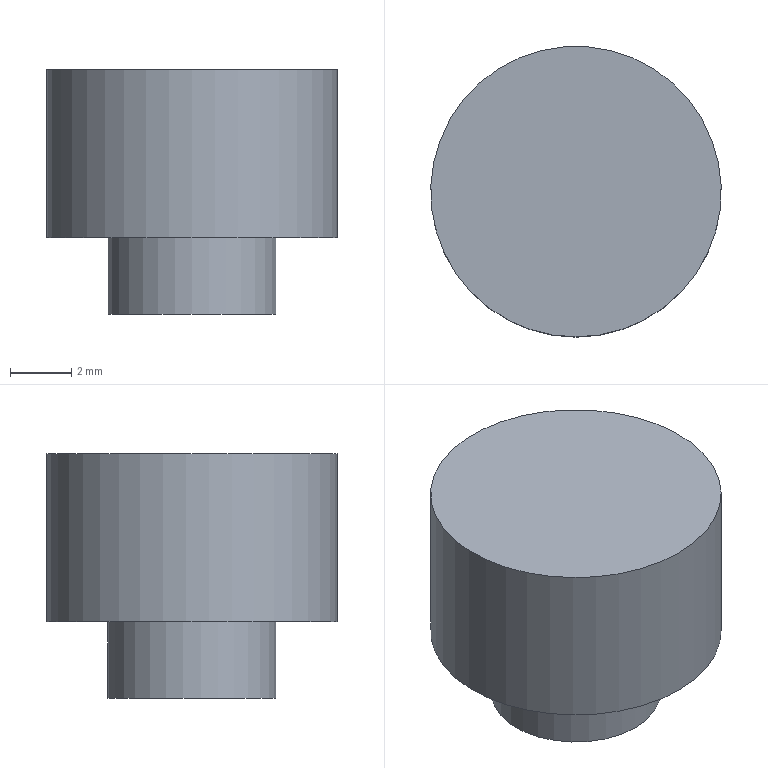Part | STEP file | SOLID | 1 solid | 5 faces | box 9.5 x 9.5 x 8 mm | volume 449.248 mm3 | plane 3 | cylinder 2 | commonest cylinder face diameters 5.5 x1 9.5 x1
STEP:
#1=CARTESIAN_POINT('',(0.,0.,0.));
#2=DIRECTION('',(0.,0.,1.));
#3=DIRECTION('',(1.,0.,0.));
#4=AXIS2_PLACEMENT_3D('',#1,#2,#3);
#5=CARTESIAN_POINT('',(0.,-2.75,-5.5));
#6=VERTEX_POINT('',#5);
#7=CARTESIAN_POINT('',(0.,0.,-5.5));
#8=DIRECTION('',(0.,0.,1.));
#9=DIRECTION('',(0.,-1.,0.));
#10=AXIS2_PLACEMENT_3D('',#7,#8,#9);
#11=CIRCLE('',#10,2.75);
#12=CARTESIAN_POINT('',(0.,0.,-5.5));
#13=DIRECTION('',(0.,0.,1.));
#14=DIRECTION('',(0.,-1.,0.));
#15=AXIS2_PLACEMENT_3D('',#12,#13,#14);
#16=PLANE('',#15);
#17=CARTESIAN_POINT('',(0.,0.));
#18=DIRECTION('',(1.,0.));
#19=AXIS2_PLACEMENT_2D('',#17,#18);
#20=CIRCLE('',#19,2.75);
#21=(GEOMETRIC_REPRESENTATION_CONTEXT(2)PARAMETRIC_REPRESENTATION_CONTEXT()REPRESENTATION_CONTEXT('',''));
#22=DEFINITIONAL_REPRESENTATION('',(#20),#21);
#23=PCURVE('',#16,#22);
#24=CARTESIAN_POINT('',(0.,0.,1.));
#25=DIRECTION('',(0.,0.,1.));
#26=DIRECTION('',(0.,-1.,0.));
#27=AXIS2_PLACEMENT_3D('',#24,#25,#26);
#28=CYLINDRICAL_SURFACE('',#27,2.75);
#29=CARTESIAN_POINT('',(0.,-6.5));
#30=DIRECTION('',(1.,0.));
#31=VECTOR('',#30,1.);
#32=LINE('',#29,#31);
#33=(GEOMETRIC_REPRESENTATION_CONTEXT(2)PARAMETRIC_REPRESENTATION_CONTEXT()REPRESENTATION_CONTEXT('',''));
#34=DEFINITIONAL_REPRESENTATION('',(#32),#33);
#35=PCURVE('',#28,#34);
#36=SURFACE_CURVE('',#11,(#23,#35),.PCURVE_S1.);
#37=EDGE_CURVE('',#6,#6,#36,.T.);
#38=ORIENTED_EDGE('',*,*,#37,.T.);
#39=EDGE_LOOP('',(#38));
#40=FACE_BOUND('',#39,.T.);
#41=CARTESIAN_POINT('',(0.,-4.75,-5.5));
#42=VERTEX_POINT('',#41);
#43=CARTESIAN_POINT('',(0.,0.,-5.5));
#44=DIRECTION('',(0.,0.,1.));
#45=DIRECTION('',(0.,-1.,0.));
#46=AXIS2_PLACEMENT_3D('',#43,#44,#45);
#47=CIRCLE('',#46,4.75);
#48=CARTESIAN_POINT('',(0.,0.));
#49=DIRECTION('',(1.,0.));
#50=AXIS2_PLACEMENT_2D('',#48,#49);
#51=CIRCLE('',#50,4.75);
#52=(GEOMETRIC_REPRESENTATION_CONTEXT(2)PARAMETRIC_REPRESENTATION_CONTEXT()REPRESENTATION_CONTEXT('',''));
#53=DEFINITIONAL_REPRESENTATION('',(#51),#52);
#54=PCURVE('',#16,#53);
#55=CARTESIAN_POINT('',(0.,0.,1.));
#56=DIRECTION('',(0.,0.,1.));
#57=DIRECTION('',(0.,-1.,0.));
#58=AXIS2_PLACEMENT_3D('',#55,#56,#57);
#59=CYLINDRICAL_SURFACE('',#58,4.75);
#60=CARTESIAN_POINT('',(0.,-6.5));
#61=DIRECTION('',(1.,0.));
#62=VECTOR('',#61,1.);
#63=LINE('',#60,#62);
#64=(GEOMETRIC_REPRESENTATION_CONTEXT(2)PARAMETRIC_REPRESENTATION_CONTEXT()REPRESENTATION_CONTEXT('',''));
#65=DEFINITIONAL_REPRESENTATION('',(#63),#64);
#66=PCURVE('',#59,#65);
#67=SURFACE_CURVE('',#47,(#54,#66),.PCURVE_S1.);
#68=EDGE_CURVE('',#42,#42,#67,.T.);
#69=ORIENTED_EDGE('',*,*,#68,.F.);
#70=EDGE_LOOP('',(#69));
#71=FACE_BOUND('',#70,.T.);
#72=ADVANCED_FACE('',(#40,#71),#16,.F.);
#73=CARTESIAN_POINT('',(0.,-4.75,0.));
#74=VERTEX_POINT('',#73);
#75=CARTESIAN_POINT('',(0.,0.,0.));
#76=DIRECTION('',(0.,0.,1.));
#77=DIRECTION('',(0.,-1.,0.));
#78=AXIS2_PLACEMENT_3D('',#75,#76,#77);
#79=CIRCLE('',#78,4.75);
#80=CARTESIAN_POINT('',(0.,0.,0.));
#81=DIRECTION('',(0.,0.,1.));
#82=DIRECTION('',(0.,-1.,0.));
#83=AXIS2_PLACEMENT_3D('',#80,#81,#82);
#84=PLANE('',#83);
#85=CARTESIAN_POINT('',(0.,0.));
#86=DIRECTION('',(1.,0.));
#87=AXIS2_PLACEMENT_2D('',#85,#86);
#88=CIRCLE('',#87,4.75);
#89=(GEOMETRIC_REPRESENTATION_CONTEXT(2)PARAMETRIC_REPRESENTATION_CONTEXT()REPRESENTATION_CONTEXT('',''));
#90=DEFINITIONAL_REPRESENTATION('',(#88),#89);
#91=PCURVE('',#84,#90);
#92=CARTESIAN_POINT('',(0.,-1.));
#93=DIRECTION('',(1.,0.));
#94=VECTOR('',#93,1.);
#95=LINE('',#92,#94);
#96=(GEOMETRIC_REPRESENTATION_CONTEXT(2)PARAMETRIC_REPRESENTATION_CONTEXT()REPRESENTATION_CONTEXT('',''));
#97=DEFINITIONAL_REPRESENTATION('',(#95),#96);
#98=PCURVE('',#59,#97);
#99=SURFACE_CURVE('',#79,(#91,#98),.PCURVE_S1.);
#100=EDGE_CURVE('',#74,#74,#99,.T.);
#101=ORIENTED_EDGE('',*,*,#100,.T.);
#102=EDGE_LOOP('',(#101));
#103=FACE_BOUND('',#102,.T.);
#104=ADVANCED_FACE('',(#103),#84,.T.);
#105=ORIENTED_EDGE('',*,*,#100,.F.);
#106=CARTESIAN_POINT('',(0.,-4.75,-5.5));
#107=CARTESIAN_POINT('',(0.,-4.75,0.));
#108=B_SPLINE_CURVE_WITH_KNOTS('',1,(#106,#107),.UNSPECIFIED.,.F.,.F.,(2,2),(-6.5,-1.),.PIECEWISE_BEZIER_KNOTS.);
#109=CARTESIAN_POINT('',(0.,0.));
#110=DIRECTION('',(0.,1.));
#111=VECTOR('',#110,1.);
#112=LINE('',#109,#111);
#113=(GEOMETRIC_REPRESENTATION_CONTEXT(2)PARAMETRIC_REPRESENTATION_CONTEXT()REPRESENTATION_CONTEXT('',''));
#114=DEFINITIONAL_REPRESENTATION('',(#112),#113);
#115=PCURVE('',#59,#114);
#116=CARTESIAN_POINT('',(6.283,0.));
#117=DIRECTION('',(0.,1.));
#118=VECTOR('',#117,1.);
#119=LINE('',#116,#118);
#120=(GEOMETRIC_REPRESENTATION_CONTEXT(2)PARAMETRIC_REPRESENTATION_CONTEXT()REPRESENTATION_CONTEXT('',''));
#121=DEFINITIONAL_REPRESENTATION('',(#119),#120);
#122=PCURVE('',#59,#121);
#123=SEAM_CURVE('',#108,(#115,#122),.PCURVE_S1.);
#124=EDGE_CURVE('',#42,#74,#123,.T.);
#125=ORIENTED_EDGE('',*,*,#124,.F.);
#126=ORIENTED_EDGE('',*,*,#68,.T.);
#127=ORIENTED_EDGE('',*,*,#124,.T.);
#128=EDGE_LOOP('',(#105,#125,#126,#127));
#129=FACE_BOUND('',#128,.T.);
#130=ADVANCED_FACE('',(#129),#59,.T.);
#131=CARTESIAN_POINT('',(0.,-2.75,-8.));
#132=VERTEX_POINT('',#131);
#133=CARTESIAN_POINT('',(0.,0.,-8.));
#134=DIRECTION('',(0.,0.,1.));
#135=DIRECTION('',(0.,-1.,0.));
#136=AXIS2_PLACEMENT_3D('',#133,#134,#135);
#137=CIRCLE('',#136,2.75);
#138=CARTESIAN_POINT('',(0.,0.,-8.));
#139=DIRECTION('',(0.,0.,1.));
#140=DIRECTION('',(0.,-1.,0.));
#141=AXIS2_PLACEMENT_3D('',#138,#139,#140);
#142=PLANE('',#141);
#143=CARTESIAN_POINT('',(0.,0.));
#144=DIRECTION('',(1.,0.));
#145=AXIS2_PLACEMENT_2D('',#143,#144);
#146=CIRCLE('',#145,2.75);
#147=(GEOMETRIC_REPRESENTATION_CONTEXT(2)PARAMETRIC_REPRESENTATION_CONTEXT()REPRESENTATION_CONTEXT('',''));
#148=DEFINITIONAL_REPRESENTATION('',(#146),#147);
#149=PCURVE('',#142,#148);
#150=CARTESIAN_POINT('',(0.,-9.));
#151=DIRECTION('',(1.,0.));
#152=VECTOR('',#151,1.);
#153=LINE('',#150,#152);
#154=(GEOMETRIC_REPRESENTATION_CONTEXT(2)PARAMETRIC_REPRESENTATION_CONTEXT()REPRESENTATION_CONTEXT('',''));
#155=DEFINITIONAL_REPRESENTATION('',(#153),#154);
#156=PCURVE('',#28,#155);
#157=SURFACE_CURVE('',#137,(#149,#156),.PCURVE_S1.);
#158=EDGE_CURVE('',#132,#132,#157,.T.);
#159=ORIENTED_EDGE('',*,*,#158,.F.);
#160=EDGE_LOOP('',(#159));
#161=FACE_BOUND('',#160,.T.);
#162=ADVANCED_FACE('',(#161),#142,.F.);
#163=ORIENTED_EDGE('',*,*,#37,.F.);
#164=CARTESIAN_POINT('',(0.,-2.75,-8.));
#165=CARTESIAN_POINT('',(0.,-2.75,-5.5));
#166=B_SPLINE_CURVE_WITH_KNOTS('',1,(#164,#165),.UNSPECIFIED.,.F.,.F.,(2,2),(-9.,-6.5),.PIECEWISE_BEZIER_KNOTS.);
#167=CARTESIAN_POINT('',(0.,0.));
#168=DIRECTION('',(0.,1.));
#169=VECTOR('',#168,1.);
#170=LINE('',#167,#169);
#171=(GEOMETRIC_REPRESENTATION_CONTEXT(2)PARAMETRIC_REPRESENTATION_CONTEXT()REPRESENTATION_CONTEXT('',''));
#172=DEFINITIONAL_REPRESENTATION('',(#170),#171);
#173=PCURVE('',#28,#172);
#174=CARTESIAN_POINT('',(6.283,0.));
#175=DIRECTION('',(0.,1.));
#176=VECTOR('',#175,1.);
#177=LINE('',#174,#176);
#178=(GEOMETRIC_REPRESENTATION_CONTEXT(2)PARAMETRIC_REPRESENTATION_CONTEXT()REPRESENTATION_CONTEXT('',''));
#179=DEFINITIONAL_REPRESENTATION('',(#177),#178);
#180=PCURVE('',#28,#179);
#181=SEAM_CURVE('',#166,(#173,#180),.PCURVE_S1.);
#182=EDGE_CURVE('',#132,#6,#181,.T.);
#183=ORIENTED_EDGE('',*,*,#182,.F.);
#184=ORIENTED_EDGE('',*,*,#158,.T.);
#185=ORIENTED_EDGE('',*,*,#182,.T.);
#186=EDGE_LOOP('',(#163,#183,#184,#185));
#187=FACE_BOUND('',#186,.T.);
#188=ADVANCED_FACE('',(#187),#28,.T.);
#189=CLOSED_SHELL('',(#72,#104,#130,#162,#188));
#190=MANIFOLD_SOLID_BREP('',#189);
#191=(LENGTH_UNIT()NAMED_UNIT(*)SI_UNIT(.MILLI.,.METRE.));
#192=UNCERTAINTY_MEASURE_WITH_UNIT(LENGTH_MEASURE(0.00001),#191,'','');
#193=(NAMED_UNIT(*)PLANE_ANGLE_UNIT()SI_UNIT($,.RADIAN.));
#194=(NAMED_UNIT(*)SI_UNIT($,.STERADIAN.)SOLID_ANGLE_UNIT());
#195=(GEOMETRIC_REPRESENTATION_CONTEXT(3)GLOBAL_UNCERTAINTY_ASSIGNED_CONTEXT((#192))GLOBAL_UNIT_ASSIGNED_CONTEXT((#191,#193,#194))REPRESENTATION_CONTEXT('',''));
#196=ADVANCED_BREP_SHAPE_REPRESENTATION('',(#4,#190),#195);